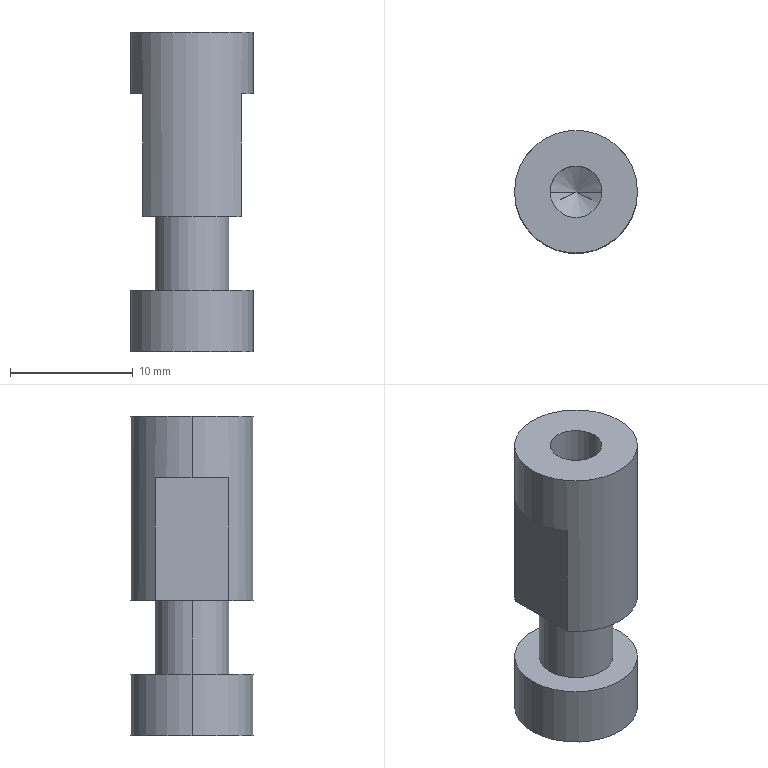Part | STEP file | 2100 Cylinder joint | 1 solid | 18 faces | box 10 x 10 x 26 mm | volume 1459 mm3 | cylinder 8 | plane 8 | cone 2 | commonest cylinder face diameters 10 x4 4.2 x2 6 x2
STEP:
#1=CARTESIAN_POINT('',(0.,0.,0.));
#2=DIRECTION('',(0.,0.,1.));
#3=DIRECTION('',(1.,0.,0.));
#4=AXIS2_PLACEMENT_3D('',#1,#2,#3);
#5=CARTESIAN_POINT('',(2.1,0.,12.));
#6=VERTEX_POINT('',#5);
#7=CARTESIAN_POINT('',(2.1,0.,26.));
#8=VERTEX_POINT('',#7);
#9=CARTESIAN_POINT('',(2.1,0.,26.));
#10=DIRECTION('',(0.,0.,1.));
#11=VECTOR('',#10,1.);
#12=LINE('',#9,#11);
#13=CARTESIAN_POINT('',(0.,0.,26.));
#14=DIRECTION('',(0.,0.,1.));
#15=DIRECTION('',(1.,0.,0.));
#16=AXIS2_PLACEMENT_3D('',#13,#14,#15);
#17=CYLINDRICAL_SURFACE('',#16,2.1);
#18=CARTESIAN_POINT('',(6.283,0.));
#19=DIRECTION('',(0.,1.));
#20=VECTOR('',#19,1.);
#21=LINE('',#18,#20);
#22=(GEOMETRIC_REPRESENTATION_CONTEXT(2)PARAMETRIC_REPRESENTATION_CONTEXT()REPRESENTATION_CONTEXT('',''));
#23=DEFINITIONAL_REPRESENTATION('',(#21),#22);
#24=PCURVE('',#17,#23);
#25=CARTESIAN_POINT('',(0.,0.,26.));
#26=DIRECTION('',(0.,0.,1.));
#27=DIRECTION('',(1.,0.,0.));
#28=AXIS2_PLACEMENT_3D('',#25,#26,#27);
#29=CYLINDRICAL_SURFACE('',#28,2.1);
#30=CARTESIAN_POINT('',(0.,0.));
#31=DIRECTION('',(0.,1.));
#32=VECTOR('',#31,1.);
#33=LINE('',#30,#32);
#34=(GEOMETRIC_REPRESENTATION_CONTEXT(2)PARAMETRIC_REPRESENTATION_CONTEXT()REPRESENTATION_CONTEXT('',''));
#35=DEFINITIONAL_REPRESENTATION('',(#33),#34);
#36=PCURVE('',#29,#35);
#37=SURFACE_CURVE('',#12,(#24,#36),.PCURVE_S1.);
#38=EDGE_CURVE('',#6,#8,#37,.T.);
#39=ORIENTED_EDGE('',*,*,#38,.T.);
#40=CARTESIAN_POINT('',(-2.1,0.,26.));
#41=VERTEX_POINT('',#40);
#42=CARTESIAN_POINT('',(0.,0.,26.));
#43=DIRECTION('',(0.,0.,1.));
#44=DIRECTION('',(1.,0.,0.));
#45=AXIS2_PLACEMENT_3D('',#42,#43,#44);
#46=CIRCLE('',#45,2.1);
#47=CARTESIAN_POINT('',(0.,0.));
#48=DIRECTION('',(1.,0.));
#49=VECTOR('',#48,1.);
#50=LINE('',#47,#49);
#51=(GEOMETRIC_REPRESENTATION_CONTEXT(2)PARAMETRIC_REPRESENTATION_CONTEXT()REPRESENTATION_CONTEXT('',''));
#52=DEFINITIONAL_REPRESENTATION('',(#50),#51);
#53=PCURVE('',#17,#52);
#54=CARTESIAN_POINT('',(0.,0.,26.));
#55=DIRECTION('',(0.,0.,1.));
#56=DIRECTION('',(1.,0.,0.));
#57=AXIS2_PLACEMENT_3D('',#54,#55,#56);
#58=PLANE('',#57);
#59=CARTESIAN_POINT('',(0.,0.));
#60=DIRECTION('',(1.,0.));
#61=AXIS2_PLACEMENT_2D('',#59,#60);
#62=CIRCLE('',#61,2.1);
#63=(GEOMETRIC_REPRESENTATION_CONTEXT(2)PARAMETRIC_REPRESENTATION_CONTEXT()REPRESENTATION_CONTEXT('',''));
#64=DEFINITIONAL_REPRESENTATION('',(#62),#63);
#65=PCURVE('',#58,#64);
#66=SURFACE_CURVE('',#46,(#53,#65),.PCURVE_S1.);
#67=EDGE_CURVE('',#41,#8,#66,.T.);
#68=ORIENTED_EDGE('',*,*,#67,.F.);
#69=CARTESIAN_POINT('',(-2.1,0.,12.));
#70=VERTEX_POINT('',#69);
#71=CARTESIAN_POINT('',(-2.1,0.,26.));
#72=DIRECTION('',(0.,0.,1.));
#73=VECTOR('',#72,1.);
#74=LINE('',#71,#73);
#75=CARTESIAN_POINT('',(3.142,0.));
#76=DIRECTION('',(0.,1.));
#77=VECTOR('',#76,1.);
#78=LINE('',#75,#77);
#79=(GEOMETRIC_REPRESENTATION_CONTEXT(2)PARAMETRIC_REPRESENTATION_CONTEXT()REPRESENTATION_CONTEXT('',''));
#80=DEFINITIONAL_REPRESENTATION('',(#78),#79);
#81=PCURVE('',#17,#80);
#82=CARTESIAN_POINT('',(3.142,0.));
#83=DIRECTION('',(0.,1.));
#84=VECTOR('',#83,1.);
#85=LINE('',#82,#84);
#86=(GEOMETRIC_REPRESENTATION_CONTEXT(2)PARAMETRIC_REPRESENTATION_CONTEXT()REPRESENTATION_CONTEXT('',''));
#87=DEFINITIONAL_REPRESENTATION('',(#85),#86);
#88=PCURVE('',#29,#87);
#89=SURFACE_CURVE('',#74,(#81,#88),.PCURVE_S1.);
#90=EDGE_CURVE('',#70,#41,#89,.T.);
#91=ORIENTED_EDGE('',*,*,#90,.F.);
#92=CARTESIAN_POINT('',(0.,0.,12.));
#93=DIRECTION('',(0.,0.,1.));
#94=DIRECTION('',(1.,0.,0.));
#95=AXIS2_PLACEMENT_3D('',#92,#93,#94);
#96=CIRCLE('',#95,2.1);
#97=CARTESIAN_POINT('',(0.,-14.));
#98=DIRECTION('',(1.,0.));
#99=VECTOR('',#98,1.);
#100=LINE('',#97,#99);
#101=(GEOMETRIC_REPRESENTATION_CONTEXT(2)PARAMETRIC_REPRESENTATION_CONTEXT()REPRESENTATION_CONTEXT('',''));
#102=DEFINITIONAL_REPRESENTATION('',(#100),#101);
#103=PCURVE('',#17,#102);
#104=CARTESIAN_POINT('',(0.,0.,12.));
#105=DIRECTION('',(0.,0.,1.));
#106=DIRECTION('',(1.,0.,0.));
#107=AXIS2_PLACEMENT_3D('',#104,#105,#106);
#108=CONICAL_SURFACE('',#107,2.1,1.03);
#109=CARTESIAN_POINT('',(0.,0.));
#110=DIRECTION('',(1.,0.));
#111=VECTOR('',#110,1.);
#112=LINE('',#109,#111);
#113=(GEOMETRIC_REPRESENTATION_CONTEXT(2)PARAMETRIC_REPRESENTATION_CONTEXT()REPRESENTATION_CONTEXT('',''));
#114=DEFINITIONAL_REPRESENTATION('',(#112),#113);
#115=PCURVE('',#108,#114);
#116=SURFACE_CURVE('',#96,(#103,#115),.PCURVE_S1.);
#117=EDGE_CURVE('',#70,#6,#116,.T.);
#118=ORIENTED_EDGE('',*,*,#117,.T.);
#119=EDGE_LOOP('',(#39,#68,#91,#118));
#120=FACE_BOUND('',#119,.F.);
#121=ADVANCED_FACE('',(#120),#17,.F.);
#122=ORIENTED_EDGE('',*,*,#117,.F.);
#123=CARTESIAN_POINT('',(0.,0.,10.738));
#124=VERTEX_POINT('',#123);
#125=CARTESIAN_POINT('',(-2.1,0.,12.));
#126=DIRECTION('',(-0.8572,0.,0.515));
#127=VECTOR('',#126,1.);
#128=LINE('',#125,#127);
#129=CARTESIAN_POINT('',(3.142,0.));
#130=DIRECTION('',(0.,1.));
#131=VECTOR('',#130,1.);
#132=LINE('',#129,#131);
#133=(GEOMETRIC_REPRESENTATION_CONTEXT(2)PARAMETRIC_REPRESENTATION_CONTEXT()REPRESENTATION_CONTEXT('',''));
#134=DEFINITIONAL_REPRESENTATION('',(#132),#133);
#135=PCURVE('',#108,#134);
#136=CARTESIAN_POINT('',(0.,0.,12.));
#137=DIRECTION('',(0.,0.,1.));
#138=DIRECTION('',(1.,0.,0.));
#139=AXIS2_PLACEMENT_3D('',#136,#137,#138);
#140=CONICAL_SURFACE('',#139,2.1,1.03);
#141=CARTESIAN_POINT('',(3.142,0.));
#142=DIRECTION('',(0.,1.));
#143=VECTOR('',#142,1.);
#144=LINE('',#141,#143);
#145=(GEOMETRIC_REPRESENTATION_CONTEXT(2)PARAMETRIC_REPRESENTATION_CONTEXT()REPRESENTATION_CONTEXT('',''));
#146=DEFINITIONAL_REPRESENTATION('',(#144),#145);
#147=PCURVE('',#140,#146);
#148=SURFACE_CURVE('',#128,(#135,#147),.PCURVE_S1.);
#149=EDGE_CURVE('',#124,#70,#148,.T.);
#150=ORIENTED_EDGE('',*,*,#149,.F.);
#151=CARTESIAN_POINT('',(2.1,0.,12.));
#152=DIRECTION('',(0.8572,0.,0.515));
#153=VECTOR('',#152,1.);
#154=LINE('',#151,#153);
#155=CARTESIAN_POINT('',(6.283,0.));
#156=DIRECTION('',(0.,1.));
#157=VECTOR('',#156,1.);
#158=LINE('',#155,#157);
#159=(GEOMETRIC_REPRESENTATION_CONTEXT(2)PARAMETRIC_REPRESENTATION_CONTEXT()REPRESENTATION_CONTEXT('',''));
#160=DEFINITIONAL_REPRESENTATION('',(#158),#159);
#161=PCURVE('',#108,#160);
#162=CARTESIAN_POINT('',(0.,0.));
#163=DIRECTION('',(0.,1.));
#164=VECTOR('',#163,1.);
#165=LINE('',#162,#164);
#166=(GEOMETRIC_REPRESENTATION_CONTEXT(2)PARAMETRIC_REPRESENTATION_CONTEXT()REPRESENTATION_CONTEXT('',''));
#167=DEFINITIONAL_REPRESENTATION('',(#165),#166);
#168=PCURVE('',#140,#167);
#169=SURFACE_CURVE('',#154,(#161,#168),.PCURVE_S1.);
#170=EDGE_CURVE('',#124,#6,#169,.T.);
#171=ORIENTED_EDGE('',*,*,#170,.T.);
#172=EDGE_LOOP('',(#122,#150,#171));
#173=FACE_BOUND('',#172,.F.);
#174=ADVANCED_FACE('',(#173),#108,.F.);
#175=CARTESIAN_POINT('',(3.,0.,11.));
#176=VERTEX_POINT('',#175);
#177=CARTESIAN_POINT('',(-3.,0.,11.));
#178=VERTEX_POINT('',#177);
#179=CARTESIAN_POINT('',(0.,0.,11.));
#180=DIRECTION('',(0.,0.,1.));
#181=DIRECTION('',(1.,0.,0.));
#182=AXIS2_PLACEMENT_3D('',#179,#180,#181);
#183=CIRCLE('',#182,3.);
#184=CARTESIAN_POINT('',(0.,0.,11.));
#185=DIRECTION('',(0.,0.,-1.));
#186=DIRECTION('',(-1.,0.,0.));
#187=AXIS2_PLACEMENT_3D('',#184,#185,#186);
#188=CYLINDRICAL_SURFACE('',#187,3.);
#189=CARTESIAN_POINT('',(3.142,0.));
#190=DIRECTION('',(-1.,0.));
#191=VECTOR('',#190,1.);
#192=LINE('',#189,#191);
#193=(GEOMETRIC_REPRESENTATION_CONTEXT(2)PARAMETRIC_REPRESENTATION_CONTEXT()REPRESENTATION_CONTEXT('',''));
#194=DEFINITIONAL_REPRESENTATION('',(#192),#193);
#195=PCURVE('',#188,#194);
#196=CARTESIAN_POINT('',(0.,0.,11.));
#197=DIRECTION('',(0.,0.,1.));
#198=DIRECTION('',(1.,0.,0.));
#199=AXIS2_PLACEMENT_3D('',#196,#197,#198);
#200=PLANE('',#199);
#201=CARTESIAN_POINT('',(0.,0.));
#202=DIRECTION('',(1.,0.));
#203=AXIS2_PLACEMENT_2D('',#201,#202);
#204=CIRCLE('',#203,3.);
#205=(GEOMETRIC_REPRESENTATION_CONTEXT(2)PARAMETRIC_REPRESENTATION_CONTEXT()REPRESENTATION_CONTEXT('',''));
#206=DEFINITIONAL_REPRESENTATION('',(#204),#205);
#207=PCURVE('',#200,#206);
#208=SURFACE_CURVE('',#183,(#195,#207),.PCURVE_S1.);
#209=EDGE_CURVE('',#176,#178,#208,.T.);
#210=ORIENTED_EDGE('',*,*,#209,.F.);
#211=CARTESIAN_POINT('',(3.,0.,5.));
#212=VERTEX_POINT('',#211);
#213=CARTESIAN_POINT('',(3.,0.,11.));
#214=DIRECTION('',(0.,0.,-1.));
#215=VECTOR('',#214,1.);
#216=LINE('',#213,#215);
#217=CARTESIAN_POINT('',(3.142,0.));
#218=DIRECTION('',(0.,1.));
#219=VECTOR('',#218,1.);
#220=LINE('',#217,#219);
#221=(GEOMETRIC_REPRESENTATION_CONTEXT(2)PARAMETRIC_REPRESENTATION_CONTEXT()REPRESENTATION_CONTEXT('',''));
#222=DEFINITIONAL_REPRESENTATION('',(#220),#221);
#223=PCURVE('',#188,#222);
#224=CARTESIAN_POINT('',(0.,0.,11.));
#225=DIRECTION('',(0.,0.,-1.));
#226=DIRECTION('',(-1.,0.,0.));
#227=AXIS2_PLACEMENT_3D('',#224,#225,#226);
#228=CYLINDRICAL_SURFACE('',#227,3.);
#229=CARTESIAN_POINT('',(3.142,0.));
#230=DIRECTION('',(0.,1.));
#231=VECTOR('',#230,1.);
#232=LINE('',#229,#231);
#233=(GEOMETRIC_REPRESENTATION_CONTEXT(2)PARAMETRIC_REPRESENTATION_CONTEXT()REPRESENTATION_CONTEXT('',''));
#234=DEFINITIONAL_REPRESENTATION('',(#232),#233);
#235=PCURVE('',#228,#234);
#236=SURFACE_CURVE('',#216,(#223,#235),.PCURVE_S1.);
#237=EDGE_CURVE('',#176,#212,#236,.T.);
#238=ORIENTED_EDGE('',*,*,#237,.T.);
#239=CARTESIAN_POINT('',(-3.,0.,5.));
#240=VERTEX_POINT('',#239);
#241=CARTESIAN_POINT('',(0.,0.,5.));
#242=DIRECTION('',(0.,0.,1.));
#243=DIRECTION('',(1.,0.,0.));
#244=AXIS2_PLACEMENT_3D('',#241,#242,#243);
#245=CIRCLE('',#244,3.);
#246=CARTESIAN_POINT('',(3.142,6.));
#247=DIRECTION('',(-1.,0.));
#248=VECTOR('',#247,1.);
#249=LINE('',#246,#248);
#250=(GEOMETRIC_REPRESENTATION_CONTEXT(2)PARAMETRIC_REPRESENTATION_CONTEXT()REPRESENTATION_CONTEXT('',''));
#251=DEFINITIONAL_REPRESENTATION('',(#249),#250);
#252=PCURVE('',#188,#251);
#253=CARTESIAN_POINT('',(0.,0.,5.));
#254=DIRECTION('',(0.,0.,1.));
#255=DIRECTION('',(1.,0.,0.));
#256=AXIS2_PLACEMENT_3D('',#253,#254,#255);
#257=PLANE('',#256);
#258=CARTESIAN_POINT('',(0.,0.));
#259=DIRECTION('',(1.,0.));
#260=AXIS2_PLACEMENT_2D('',#258,#259);
#261=CIRCLE('',#260,3.);
#262=(GEOMETRIC_REPRESENTATION_CONTEXT(2)PARAMETRIC_REPRESENTATION_CONTEXT()REPRESENTATION_CONTEXT('',''));
#263=DEFINITIONAL_REPRESENTATION('',(#261),#262);
#264=PCURVE('',#257,#263);
#265=SURFACE_CURVE('',#245,(#252,#264),.PCURVE_S1.);
#266=EDGE_CURVE('',#212,#240,#265,.T.);
#267=ORIENTED_EDGE('',*,*,#266,.T.);
#268=CARTESIAN_POINT('',(-3.,0.,11.));
#269=DIRECTION('',(0.,0.,-1.));
#270=VECTOR('',#269,1.);
#271=LINE('',#268,#270);
#272=CARTESIAN_POINT('',(0.,0.));
#273=DIRECTION('',(0.,1.));
#274=VECTOR('',#273,1.);
#275=LINE('',#272,#274);
#276=(GEOMETRIC_REPRESENTATION_CONTEXT(2)PARAMETRIC_REPRESENTATION_CONTEXT()REPRESENTATION_CONTEXT('',''));
#277=DEFINITIONAL_REPRESENTATION('',(#275),#276);
#278=PCURVE('',#188,#277);
#279=CARTESIAN_POINT('',(6.283,0.));
#280=DIRECTION('',(0.,1.));
#281=VECTOR('',#280,1.);
#282=LINE('',#279,#281);
#283=(GEOMETRIC_REPRESENTATION_CONTEXT(2)PARAMETRIC_REPRESENTATION_CONTEXT()REPRESENTATION_CONTEXT('',''));
#284=DEFINITIONAL_REPRESENTATION('',(#282),#283);
#285=PCURVE('',#228,#284);
#286=SURFACE_CURVE('',#271,(#278,#285),.PCURVE_S1.);
#287=EDGE_CURVE('',#178,#240,#286,.T.);
#288=ORIENTED_EDGE('',*,*,#287,.F.);
#289=EDGE_LOOP('',(#210,#238,#267,#288));
#290=FACE_BOUND('',#289,.T.);
#291=ADVANCED_FACE('',(#290),#188,.T.);
#292=CARTESIAN_POINT('',(5.,0.,5.));
#293=VERTEX_POINT('',#292);
#294=CARTESIAN_POINT('',(-5.,0.,5.));
#295=VERTEX_POINT('',#294);
#296=CARTESIAN_POINT('',(0.,0.,5.));
#297=DIRECTION('',(0.,0.,1.));
#298=DIRECTION('',(1.,0.,0.));
#299=AXIS2_PLACEMENT_3D('',#296,#297,#298);
#300=CIRCLE('',#299,5.);
#301=CARTESIAN_POINT('',(0.,0.,5.));
#302=DIRECTION('',(0.,0.,-1.));
#303=DIRECTION('',(-1.,0.,0.));
#304=AXIS2_PLACEMENT_3D('',#301,#302,#303);
#305=CYLINDRICAL_SURFACE('',#304,5.);
#306=CARTESIAN_POINT('',(3.142,0.));
#307=DIRECTION('',(-1.,0.));
#308=VECTOR('',#307,1.);
#309=LINE('',#306,#308);
#310=(GEOMETRIC_REPRESENTATION_CONTEXT(2)PARAMETRIC_REPRESENTATION_CONTEXT()REPRESENTATION_CONTEXT('',''));
#311=DEFINITIONAL_REPRESENTATION('',(#309),#310);
#312=PCURVE('',#305,#311);
#313=CARTESIAN_POINT('',(0.,0.));
#314=DIRECTION('',(1.,0.));
#315=AXIS2_PLACEMENT_2D('',#313,#314);
#316=CIRCLE('',#315,5.);
#317=(GEOMETRIC_REPRESENTATION_CONTEXT(2)PARAMETRIC_REPRESENTATION_CONTEXT()REPRESENTATION_CONTEXT('',''));
#318=DEFINITIONAL_REPRESENTATION('',(#316),#317);
#319=PCURVE('',#257,#318);
#320=SURFACE_CURVE('',#300,(#312,#319),.PCURVE_S1.);
#321=EDGE_CURVE('',#293,#295,#320,.T.);
#322=ORIENTED_EDGE('',*,*,#321,.F.);
#323=CARTESIAN_POINT('',(5.,0.,0.));
#324=VERTEX_POINT('',#323);
#325=CARTESIAN_POINT('',(5.,0.,5.));
#326=DIRECTION('',(0.,0.,-1.));
#327=VECTOR('',#326,1.);
#328=LINE('',#325,#327);
#329=CARTESIAN_POINT('',(3.142,0.));
#330=DIRECTION('',(0.,1.));
#331=VECTOR('',#330,1.);
#332=LINE('',#329,#331);
#333=(GEOMETRIC_REPRESENTATION_CONTEXT(2)PARAMETRIC_REPRESENTATION_CONTEXT()REPRESENTATION_CONTEXT('',''));
#334=DEFINITIONAL_REPRESENTATION('',(#332),#333);
#335=PCURVE('',#305,#334);
#336=CARTESIAN_POINT('',(0.,0.,5.));
#337=DIRECTION('',(0.,0.,-1.));
#338=DIRECTION('',(-1.,0.,0.));
#339=AXIS2_PLACEMENT_3D('',#336,#337,#338);
#340=CYLINDRICAL_SURFACE('',#339,5.);
#341=CARTESIAN_POINT('',(3.142,0.));
#342=DIRECTION('',(0.,1.));
#343=VECTOR('',#342,1.);
#344=LINE('',#341,#343);
#345=(GEOMETRIC_REPRESENTATION_CONTEXT(2)PARAMETRIC_REPRESENTATION_CONTEXT()REPRESENTATION_CONTEXT('',''));
#346=DEFINITIONAL_REPRESENTATION('',(#344),#345);
#347=PCURVE('',#340,#346);
#348=SURFACE_CURVE('',#328,(#335,#347),.PCURVE_S1.);
#349=EDGE_CURVE('',#293,#324,#348,.T.);
#350=ORIENTED_EDGE('',*,*,#349,.T.);
#351=CARTESIAN_POINT('',(-5.,0.,0.));
#352=VERTEX_POINT('',#351);
#353=CARTESIAN_POINT('',(0.,0.,0.));
#354=DIRECTION('',(0.,0.,1.));
#355=DIRECTION('',(1.,0.,0.));
#356=AXIS2_PLACEMENT_3D('',#353,#354,#355);
#357=CIRCLE('',#356,5.);
#358=CARTESIAN_POINT('',(3.142,5.));
#359=DIRECTION('',(-1.,0.));
#360=VECTOR('',#359,1.);
#361=LINE('',#358,#360);
#362=(GEOMETRIC_REPRESENTATION_CONTEXT(2)PARAMETRIC_REPRESENTATION_CONTEXT()REPRESENTATION_CONTEXT('',''));
#363=DEFINITIONAL_REPRESENTATION('',(#361),#362);
#364=PCURVE('',#305,#363);
#365=CARTESIAN_POINT('',(0.,0.,0.));
#366=DIRECTION('',(0.,0.,1.));
#367=DIRECTION('',(1.,0.,0.));
#368=AXIS2_PLACEMENT_3D('',#365,#366,#367);
#369=PLANE('',#368);
#370=CARTESIAN_POINT('',(0.,0.));
#371=DIRECTION('',(1.,0.));
#372=AXIS2_PLACEMENT_2D('',#370,#371);
#373=CIRCLE('',#372,5.);
#374=(GEOMETRIC_REPRESENTATION_CONTEXT(2)PARAMETRIC_REPRESENTATION_CONTEXT()REPRESENTATION_CONTEXT('',''));
#375=DEFINITIONAL_REPRESENTATION('',(#373),#374);
#376=PCURVE('',#369,#375);
#377=SURFACE_CURVE('',#357,(#364,#376),.PCURVE_S1.);
#378=EDGE_CURVE('',#324,#352,#377,.T.);
#379=ORIENTED_EDGE('',*,*,#378,.T.);
#380=CARTESIAN_POINT('',(-5.,0.,5.));
#381=DIRECTION('',(0.,0.,-1.));
#382=VECTOR('',#381,1.);
#383=LINE('',#380,#382);
#384=CARTESIAN_POINT('',(0.,0.));
#385=DIRECTION('',(0.,1.));
#386=VECTOR('',#385,1.);
#387=LINE('',#384,#386);
#388=(GEOMETRIC_REPRESENTATION_CONTEXT(2)PARAMETRIC_REPRESENTATION_CONTEXT()REPRESENTATION_CONTEXT('',''));
#389=DEFINITIONAL_REPRESENTATION('',(#387),#388);
#390=PCURVE('',#305,#389);
#391=CARTESIAN_POINT('',(6.283,0.));
#392=DIRECTION('',(0.,1.));
#393=VECTOR('',#392,1.);
#394=LINE('',#391,#393);
#395=(GEOMETRIC_REPRESENTATION_CONTEXT(2)PARAMETRIC_REPRESENTATION_CONTEXT()REPRESENTATION_CONTEXT('',''));
#396=DEFINITIONAL_REPRESENTATION('',(#394),#395);
#397=PCURVE('',#340,#396);
#398=SURFACE_CURVE('',#383,(#390,#397),.PCURVE_S1.);
#399=EDGE_CURVE('',#295,#352,#398,.T.);
#400=ORIENTED_EDGE('',*,*,#399,.F.);
#401=EDGE_LOOP('',(#322,#350,#379,#400));
#402=FACE_BOUND('',#401,.T.);
#403=ADVANCED_FACE('',(#402),#305,.T.);
#404=CARTESIAN_POINT('',(5.,0.,26.));
#405=VERTEX_POINT('',#404);
#406=CARTESIAN_POINT('',(-5.,0.,26.));
#407=VERTEX_POINT('',#406);
#408=CARTESIAN_POINT('',(0.,0.,26.));
#409=DIRECTION('',(0.,0.,1.));
#410=DIRECTION('',(1.,0.,0.));
#411=AXIS2_PLACEMENT_3D('',#408,#409,#410);
#412=CIRCLE('',#411,5.);
#413=CARTESIAN_POINT('',(0.,0.,26.));
#414=DIRECTION('',(0.,0.,-1.));
#415=DIRECTION('',(-1.,0.,0.));
#416=AXIS2_PLACEMENT_3D('',#413,#414,#415);
#417=CYLINDRICAL_SURFACE('',#416,5.);
#418=CARTESIAN_POINT('',(3.142,0.));
#419=DIRECTION('',(-1.,0.));
#420=VECTOR('',#419,1.);
#421=LINE('',#418,#420);
#422=(GEOMETRIC_REPRESENTATION_CONTEXT(2)PARAMETRIC_REPRESENTATION_CONTEXT()REPRESENTATION_CONTEXT('',''));
#423=DEFINITIONAL_REPRESENTATION('',(#421),#422);
#424=PCURVE('',#417,#423);
#425=CARTESIAN_POINT('',(0.,0.));
#426=DIRECTION('',(1.,0.));
#427=AXIS2_PLACEMENT_2D('',#425,#426);
#428=CIRCLE('',#427,5.);
#429=(GEOMETRIC_REPRESENTATION_CONTEXT(2)PARAMETRIC_REPRESENTATION_CONTEXT()REPRESENTATION_CONTEXT('',''));
#430=DEFINITIONAL_REPRESENTATION('',(#428),#429);
#431=PCURVE('',#58,#430);
#432=SURFACE_CURVE('',#412,(#424,#431),.PCURVE_S1.);
#433=EDGE_CURVE('',#405,#407,#432,.T.);
#434=ORIENTED_EDGE('',*,*,#433,.F.);
#435=CARTESIAN_POINT('',(5.,0.,21.));
#436=VERTEX_POINT('',#435);
#437=CARTESIAN_POINT('',(5.,0.,26.));
#438=DIRECTION('',(0.,0.,-1.));
#439=VECTOR('',#438,1.);
#440=LINE('',#437,#439);
#441=CARTESIAN_POINT('',(3.142,0.));
#442=DIRECTION('',(0.,1.));
#443=VECTOR('',#442,1.);
#444=LINE('',#441,#443);
#445=(GEOMETRIC_REPRESENTATION_CONTEXT(2)PARAMETRIC_REPRESENTATION_CONTEXT()REPRESENTATION_CONTEXT('',''));
#446=DEFINITIONAL_REPRESENTATION('',(#444),#445);
#447=PCURVE('',#417,#446);
#448=CARTESIAN_POINT('',(0.,0.,26.));
#449=DIRECTION('',(0.,0.,-1.));
#450=DIRECTION('',(-1.,0.,0.));
#451=AXIS2_PLACEMENT_3D('',#448,#449,#450);
#452=CYLINDRICAL_SURFACE('',#451,5.);
#453=CARTESIAN_POINT('',(3.142,0.));
#454=DIRECTION('',(0.,1.));
#455=VECTOR('',#454,1.);
#456=LINE('',#453,#455);
#457=(GEOMETRIC_REPRESENTATION_CONTEXT(2)PARAMETRIC_REPRESENTATION_CONTEXT()REPRESENTATION_CONTEXT('',''));
#458=DEFINITIONAL_REPRESENTATION('',(#456),#457);
#459=PCURVE('',#452,#458);
#460=SURFACE_CURVE('',#440,(#447,#459),.PCURVE_S1.);
#461=EDGE_CURVE('',#405,#436,#460,.T.);
#462=ORIENTED_EDGE('',*,*,#461,.T.);
#463=CARTESIAN_POINT('',(4.,3.,21.));
#464=VERTEX_POINT('',#463);
#465=CARTESIAN_POINT('',(0.,0.,21.));
#466=DIRECTION('',(0.,0.,-1.));
#467=DIRECTION('',(-1.,0.,0.));
#468=AXIS2_PLACEMENT_3D('',#465,#466,#467);
#469=CIRCLE('',#468,5.);
#470=CARTESIAN_POINT('',(0.,5.));
#471=DIRECTION('',(1.,0.));
#472=VECTOR('',#471,1.);
#473=LINE('',#470,#472);
#474=(GEOMETRIC_REPRESENTATION_CONTEXT(2)PARAMETRIC_REPRESENTATION_CONTEXT()REPRESENTATION_CONTEXT('',''));
#475=DEFINITIONAL_REPRESENTATION('',(#473),#474);
#476=PCURVE('',#417,#475);
#477=CARTESIAN_POINT('',(11.893,50.,21.));
#478=DIRECTION('',(0.,0.,-1.));
#479=DIRECTION('',(-1.,0.,0.));
#480=AXIS2_PLACEMENT_3D('',#477,#478,#479);
#481=PLANE('',#480);
#482=CARTESIAN_POINT('',(11.893,-50.));
#483=DIRECTION('',(1.,0.));
#484=AXIS2_PLACEMENT_2D('',#482,#483);
#485=CIRCLE('',#484,5.);
#486=(GEOMETRIC_REPRESENTATION_CONTEXT(2)PARAMETRIC_REPRESENTATION_CONTEXT()REPRESENTATION_CONTEXT('',''));
#487=DEFINITIONAL_REPRESENTATION('',(#485),#486);
#488=PCURVE('',#481,#487);
#489=SURFACE_CURVE('',#469,(#476,#488),.PCURVE_S1.);
#490=EDGE_CURVE('',#464,#436,#489,.T.);
#491=ORIENTED_EDGE('',*,*,#490,.F.);
#492=CARTESIAN_POINT('',(4.,3.,11.));
#493=VERTEX_POINT('',#492);
#494=CARTESIAN_POINT('',(4.,3.,26.));
#495=DIRECTION('',(0.,0.,1.));
#496=VECTOR('',#495,1.);
#497=LINE('',#494,#496);
#498=CARTESIAN_POINT('',(2.498,0.));
#499=DIRECTION('',(0.,-1.));
#500=VECTOR('',#499,1.);
#501=LINE('',#498,#500);
#502=(GEOMETRIC_REPRESENTATION_CONTEXT(2)PARAMETRIC_REPRESENTATION_CONTEXT()REPRESENTATION_CONTEXT('',''));
#503=DEFINITIONAL_REPRESENTATION('',(#501),#502);
#504=PCURVE('',#417,#503);
#505=CARTESIAN_POINT('',(4.,50.,9.));
#506=DIRECTION('',(1.,0.,0.));
#507=DIRECTION('',(0.,0.,-1.));
#508=AXIS2_PLACEMENT_3D('',#505,#506,#507);
#509=PLANE('',#508);
#510=CARTESIAN_POINT('',(-17.,-47.));
#511=DIRECTION('',(-1.,0.));
#512=VECTOR('',#511,1.);
#513=LINE('',#510,#512);
#514=(GEOMETRIC_REPRESENTATION_CONTEXT(2)PARAMETRIC_REPRESENTATION_CONTEXT()REPRESENTATION_CONTEXT('',''));
#515=DEFINITIONAL_REPRESENTATION('',(#513),#514);
#516=PCURVE('',#509,#515);
#517=SURFACE_CURVE('',#497,(#504,#516),.PCURVE_S1.);
#518=EDGE_CURVE('',#493,#464,#517,.T.);
#519=ORIENTED_EDGE('',*,*,#518,.F.);
#520=CARTESIAN_POINT('',(-4.,3.,11.));
#521=VERTEX_POINT('',#520);
#522=CARTESIAN_POINT('',(0.,0.,11.));
#523=DIRECTION('',(0.,0.,1.));
#524=DIRECTION('',(1.,0.,0.));
#525=AXIS2_PLACEMENT_3D('',#522,#523,#524);
#526=CIRCLE('',#525,5.);
#527=CARTESIAN_POINT('',(3.142,15.));
#528=DIRECTION('',(-1.,0.));
#529=VECTOR('',#528,1.);
#530=LINE('',#527,#529);
#531=(GEOMETRIC_REPRESENTATION_CONTEXT(2)PARAMETRIC_REPRESENTATION_CONTEXT()REPRESENTATION_CONTEXT('',''));
#532=DEFINITIONAL_REPRESENTATION('',(#530),#531);
#533=PCURVE('',#417,#532);
#534=CARTESIAN_POINT('',(0.,0.));
#535=DIRECTION('',(1.,0.));
#536=AXIS2_PLACEMENT_2D('',#534,#535);
#537=CIRCLE('',#536,5.);
#538=(GEOMETRIC_REPRESENTATION_CONTEXT(2)PARAMETRIC_REPRESENTATION_CONTEXT()REPRESENTATION_CONTEXT('',''));
#539=DEFINITIONAL_REPRESENTATION('',(#537),#538);
#540=PCURVE('',#200,#539);
#541=SURFACE_CURVE('',#526,(#533,#540),.PCURVE_S1.);
#542=EDGE_CURVE('',#493,#521,#541,.T.);
#543=ORIENTED_EDGE('',*,*,#542,.T.);
#544=CARTESIAN_POINT('',(-4.,3.,21.));
#545=VERTEX_POINT('',#544);
#546=CARTESIAN_POINT('',(-4.,3.,26.));
#547=DIRECTION('',(0.,0.,-1.));
#548=VECTOR('',#547,1.);
#549=LINE('',#546,#548);
#550=CARTESIAN_POINT('',(0.6435,0.));
#551=DIRECTION('',(0.,1.));
#552=VECTOR('',#551,1.);
#553=LINE('',#550,#552);
#554=(GEOMETRIC_REPRESENTATION_CONTEXT(2)PARAMETRIC_REPRESENTATION_CONTEXT()REPRESENTATION_CONTEXT('',''));
#555=DEFINITIONAL_REPRESENTATION('',(#553),#554);
#556=PCURVE('',#417,#555);
#557=CARTESIAN_POINT('',(-4.,50.,9.));
#558=DIRECTION('',(-1.,0.,0.));
#559=DIRECTION('',(0.,0.,1.));
#560=AXIS2_PLACEMENT_3D('',#557,#558,#559);
#561=PLANE('',#560);
#562=CARTESIAN_POINT('',(17.,-47.));
#563=DIRECTION('',(-1.,0.));
#564=VECTOR('',#563,1.);
#565=LINE('',#562,#564);
#566=(GEOMETRIC_REPRESENTATION_CONTEXT(2)PARAMETRIC_REPRESENTATION_CONTEXT()REPRESENTATION_CONTEXT('',''));
#567=DEFINITIONAL_REPRESENTATION('',(#565),#566);
#568=PCURVE('',#561,#567);
#569=SURFACE_CURVE('',#549,(#556,#568),.PCURVE_S1.);
#570=EDGE_CURVE('',#545,#521,#569,.T.);
#571=ORIENTED_EDGE('',*,*,#570,.F.);
#572=CARTESIAN_POINT('',(-5.,0.,21.));
#573=VERTEX_POINT('',#572);
#574=CARTESIAN_POINT('',(0.,0.,21.));
#575=DIRECTION('',(0.,0.,-1.));
#576=DIRECTION('',(-1.,0.,0.));
#577=AXIS2_PLACEMENT_3D('',#574,#575,#576);
#578=CIRCLE('',#577,5.);
#579=CARTESIAN_POINT('',(0.,5.));
#580=DIRECTION('',(1.,0.));
#581=VECTOR('',#580,1.);
#582=LINE('',#579,#581);
#583=(GEOMETRIC_REPRESENTATION_CONTEXT(2)PARAMETRIC_REPRESENTATION_CONTEXT()REPRESENTATION_CONTEXT('',''));
#584=DEFINITIONAL_REPRESENTATION('',(#582),#583);
#585=PCURVE('',#417,#584);
#586=CARTESIAN_POINT('',(-11.893,50.,21.));
#587=DIRECTION('',(0.,0.,-1.));
#588=DIRECTION('',(-1.,0.,0.));
#589=AXIS2_PLACEMENT_3D('',#586,#587,#588);
#590=PLANE('',#589);
#591=CARTESIAN_POINT('',(-11.893,-50.));
#592=DIRECTION('',(1.,0.));
#593=AXIS2_PLACEMENT_2D('',#591,#592);
#594=CIRCLE('',#593,5.);
#595=(GEOMETRIC_REPRESENTATION_CONTEXT(2)PARAMETRIC_REPRESENTATION_CONTEXT()REPRESENTATION_CONTEXT('',''));
#596=DEFINITIONAL_REPRESENTATION('',(#594),#595);
#597=PCURVE('',#590,#596);
#598=SURFACE_CURVE('',#578,(#585,#597),.PCURVE_S1.);
#599=EDGE_CURVE('',#573,#545,#598,.T.);
#600=ORIENTED_EDGE('',*,*,#599,.F.);
#601=CARTESIAN_POINT('',(-5.,0.,26.));
#602=DIRECTION('',(0.,0.,-1.));
#603=VECTOR('',#602,1.);
#604=LINE('',#601,#603);
#605=CARTESIAN_POINT('',(0.,0.));
#606=DIRECTION('',(0.,1.));
#607=VECTOR('',#606,1.);
#608=LINE('',#605,#607);
#609=(GEOMETRIC_REPRESENTATION_CONTEXT(2)PARAMETRIC_REPRESENTATION_CONTEXT()REPRESENTATION_CONTEXT('',''));
#610=DEFINITIONAL_REPRESENTATION('',(#608),#609);
#611=PCURVE('',#417,#610);
#612=CARTESIAN_POINT('',(6.283,0.));
#613=DIRECTION('',(0.,1.));
#614=VECTOR('',#613,1.);
#615=LINE('',#612,#614);
#616=(GEOMETRIC_REPRESENTATION_CONTEXT(2)PARAMETRIC_REPRESENTATION_CONTEXT()REPRESENTATION_CONTEXT('',''));
#617=DEFINITIONAL_REPRESENTATION('',(#615),#616);
#618=PCURVE('',#452,#617);
#619=SURFACE_CURVE('',#604,(#611,#618),.PCURVE_S1.);
#620=EDGE_CURVE('',#407,#573,#619,.T.);
#621=ORIENTED_EDGE('',*,*,#620,.F.);
#622=EDGE_LOOP('',(#434,#462,#491,#519,#543,#571,#600,#621));
#623=FACE_BOUND('',#622,.T.);
#624=ADVANCED_FACE('',(#623),#417,.T.);
#625=CARTESIAN_POINT('',(0.,0.,11.));
#626=DIRECTION('',(0.,0.,1.));
#627=DIRECTION('',(1.,0.,0.));
#628=AXIS2_PLACEMENT_3D('',#625,#626,#627);
#629=CIRCLE('',#628,3.);
#630=CARTESIAN_POINT('',(0.,0.));
#631=DIRECTION('',(1.,0.));
#632=AXIS2_PLACEMENT_2D('',#630,#631);
#633=CIRCLE('',#632,3.);
#634=(GEOMETRIC_REPRESENTATION_CONTEXT(2)PARAMETRIC_REPRESENTATION_CONTEXT()REPRESENTATION_CONTEXT('',''));
#635=DEFINITIONAL_REPRESENTATION('',(#633),#634);
#636=PCURVE('',#200,#635);
#637=CARTESIAN_POINT('',(9.425,0.));
#638=DIRECTION('',(-1.,0.));
#639=VECTOR('',#638,1.);
#640=LINE('',#637,#639);
#641=(GEOMETRIC_REPRESENTATION_CONTEXT(2)PARAMETRIC_REPRESENTATION_CONTEXT()REPRESENTATION_CONTEXT('',''));
#642=DEFINITIONAL_REPRESENTATION('',(#640),#641);
#643=PCURVE('',#228,#642);
#644=SURFACE_CURVE('',#629,(#636,#643),.PCURVE_S1.);
#645=EDGE_CURVE('',#178,#176,#644,.T.);
#646=ORIENTED_EDGE('',*,*,#645,.T.);
#647=ORIENTED_EDGE('',*,*,#209,.T.);
#648=EDGE_LOOP('',(#646,#647));
#649=FACE_BOUND('',#648,.T.);
#650=CARTESIAN_POINT('',(4.,-3.,11.));
#651=VERTEX_POINT('',#650);
#652=CARTESIAN_POINT('',(4.,0.,11.));
#653=DIRECTION('',(0.,1.,0.));
#654=VECTOR('',#653,1.);
#655=LINE('',#652,#654);
#656=CARTESIAN_POINT('',(4.,0.));
#657=DIRECTION('',(0.,1.));
#658=VECTOR('',#657,1.);
#659=LINE('',#656,#658);
#660=(GEOMETRIC_REPRESENTATION_CONTEXT(2)PARAMETRIC_REPRESENTATION_CONTEXT()REPRESENTATION_CONTEXT('',''));
#661=DEFINITIONAL_REPRESENTATION('',(#659),#660);
#662=PCURVE('',#200,#661);
#663=CARTESIAN_POINT('',(-2.,-50.));
#664=DIRECTION('',(0.,1.));
#665=VECTOR('',#664,1.);
#666=LINE('',#663,#665);
#667=(GEOMETRIC_REPRESENTATION_CONTEXT(2)PARAMETRIC_REPRESENTATION_CONTEXT()REPRESENTATION_CONTEXT('',''));
#668=DEFINITIONAL_REPRESENTATION('',(#666),#667);
#669=PCURVE('',#509,#668);
#670=SURFACE_CURVE('',#655,(#662,#669),.PCURVE_S1.);
#671=EDGE_CURVE('',#651,#493,#670,.T.);
#672=ORIENTED_EDGE('',*,*,#671,.F.);
#673=CARTESIAN_POINT('',(-4.,-3.,11.));
#674=VERTEX_POINT('',#673);
#675=CARTESIAN_POINT('',(0.,0.,11.));
#676=DIRECTION('',(0.,0.,1.));
#677=DIRECTION('',(1.,0.,0.));
#678=AXIS2_PLACEMENT_3D('',#675,#676,#677);
#679=CIRCLE('',#678,5.);
#680=CARTESIAN_POINT('',(0.,0.));
#681=DIRECTION('',(1.,0.));
#682=AXIS2_PLACEMENT_2D('',#680,#681);
#683=CIRCLE('',#682,5.);
#684=(GEOMETRIC_REPRESENTATION_CONTEXT(2)PARAMETRIC_REPRESENTATION_CONTEXT()REPRESENTATION_CONTEXT('',''));
#685=DEFINITIONAL_REPRESENTATION('',(#683),#684);
#686=PCURVE('',#200,#685);
#687=CARTESIAN_POINT('',(9.425,15.));
#688=DIRECTION('',(-1.,0.));
#689=VECTOR('',#688,1.);
#690=LINE('',#687,#689);
#691=(GEOMETRIC_REPRESENTATION_CONTEXT(2)PARAMETRIC_REPRESENTATION_CONTEXT()REPRESENTATION_CONTEXT('',''));
#692=DEFINITIONAL_REPRESENTATION('',(#690),#691);
#693=PCURVE('',#452,#692);
#694=SURFACE_CURVE('',#679,(#686,#693),.PCURVE_S1.);
#695=EDGE_CURVE('',#674,#651,#694,.T.);
#696=ORIENTED_EDGE('',*,*,#695,.F.);
#697=CARTESIAN_POINT('',(-4.,0.,11.));
#698=DIRECTION('',(0.,-1.,0.));
#699=VECTOR('',#698,1.);
#700=LINE('',#697,#699);
#701=CARTESIAN_POINT('',(-4.,0.));
#702=DIRECTION('',(0.,-1.));
#703=VECTOR('',#702,1.);
#704=LINE('',#701,#703);
#705=(GEOMETRIC_REPRESENTATION_CONTEXT(2)PARAMETRIC_REPRESENTATION_CONTEXT()REPRESENTATION_CONTEXT('',''));
#706=DEFINITIONAL_REPRESENTATION('',(#704),#705);
#707=PCURVE('',#200,#706);
#708=CARTESIAN_POINT('',(2.,-50.));
#709=DIRECTION('',(0.,-1.));
#710=VECTOR('',#709,1.);
#711=LINE('',#708,#710);
#712=(GEOMETRIC_REPRESENTATION_CONTEXT(2)PARAMETRIC_REPRESENTATION_CONTEXT()REPRESENTATION_CONTEXT('',''));
#713=DEFINITIONAL_REPRESENTATION('',(#711),#712);
#714=PCURVE('',#561,#713);
#715=SURFACE_CURVE('',#700,(#707,#714),.PCURVE_S1.);
#716=EDGE_CURVE('',#521,#674,#715,.T.);
#717=ORIENTED_EDGE('',*,*,#716,.F.);
#718=ORIENTED_EDGE('',*,*,#542,.F.);
#719=EDGE_LOOP('',(#672,#696,#717,#718));
#720=FACE_BOUND('',#719,.T.);
#721=ADVANCED_FACE('',(#649,#720),#200,.F.);
#722=ORIENTED_EDGE('',*,*,#461,.F.);
#723=CARTESIAN_POINT('',(0.,0.,26.));
#724=DIRECTION('',(0.,0.,1.));
#725=DIRECTION('',(1.,0.,0.));
#726=AXIS2_PLACEMENT_3D('',#723,#724,#725);
#727=CIRCLE('',#726,5.);
#728=CARTESIAN_POINT('',(9.425,0.));
#729=DIRECTION('',(-1.,0.));
#730=VECTOR('',#729,1.);
#731=LINE('',#728,#730);
#732=(GEOMETRIC_REPRESENTATION_CONTEXT(2)PARAMETRIC_REPRESENTATION_CONTEXT()REPRESENTATION_CONTEXT('',''));
#733=DEFINITIONAL_REPRESENTATION('',(#731),#732);
#734=PCURVE('',#452,#733);
#735=CARTESIAN_POINT('',(0.,0.));
#736=DIRECTION('',(1.,0.));
#737=AXIS2_PLACEMENT_2D('',#735,#736);
#738=CIRCLE('',#737,5.);
#739=(GEOMETRIC_REPRESENTATION_CONTEXT(2)PARAMETRIC_REPRESENTATION_CONTEXT()REPRESENTATION_CONTEXT('',''));
#740=DEFINITIONAL_REPRESENTATION('',(#738),#739);
#741=PCURVE('',#58,#740);
#742=SURFACE_CURVE('',#727,(#734,#741),.PCURVE_S1.);
#743=EDGE_CURVE('',#407,#405,#742,.T.);
#744=ORIENTED_EDGE('',*,*,#743,.F.);
#745=ORIENTED_EDGE('',*,*,#620,.T.);
#746=CARTESIAN_POINT('',(-4.,-3.,21.));
#747=VERTEX_POINT('',#746);
#748=CARTESIAN_POINT('',(0.,0.,21.));
#749=DIRECTION('',(0.,0.,-1.));
#750=DIRECTION('',(-1.,0.,0.));
#751=AXIS2_PLACEMENT_3D('',#748,#749,#750);
#752=CIRCLE('',#751,5.);
#753=CARTESIAN_POINT('',(0.,5.));
#754=DIRECTION('',(1.,0.));
#755=VECTOR('',#754,1.);
#756=LINE('',#753,#755);
#757=(GEOMETRIC_REPRESENTATION_CONTEXT(2)PARAMETRIC_REPRESENTATION_CONTEXT()REPRESENTATION_CONTEXT('',''));
#758=DEFINITIONAL_REPRESENTATION('',(#756),#757);
#759=PCURVE('',#452,#758);
#760=CARTESIAN_POINT('',(-11.893,-50.));
#761=DIRECTION('',(1.,0.));
#762=AXIS2_PLACEMENT_2D('',#760,#761);
#763=CIRCLE('',#762,5.);
#764=(GEOMETRIC_REPRESENTATION_CONTEXT(2)PARAMETRIC_REPRESENTATION_CONTEXT()REPRESENTATION_CONTEXT('',''));
#765=DEFINITIONAL_REPRESENTATION('',(#763),#764);
#766=PCURVE('',#590,#765);
#767=SURFACE_CURVE('',#752,(#759,#766),.PCURVE_S1.);
#768=EDGE_CURVE('',#747,#573,#767,.T.);
#769=ORIENTED_EDGE('',*,*,#768,.F.);
#770=CARTESIAN_POINT('',(-4.,-3.,26.));
#771=DIRECTION('',(0.,0.,1.));
#772=VECTOR('',#771,1.);
#773=LINE('',#770,#772);
#774=CARTESIAN_POINT('',(5.64,0.));
#775=DIRECTION('',(0.,-1.));
#776=VECTOR('',#775,1.);
#777=LINE('',#774,#776);
#778=(GEOMETRIC_REPRESENTATION_CONTEXT(2)PARAMETRIC_REPRESENTATION_CONTEXT()REPRESENTATION_CONTEXT('',''));
#779=DEFINITIONAL_REPRESENTATION('',(#777),#778);
#780=PCURVE('',#452,#779);
#781=CARTESIAN_POINT('',(17.,-53.));
#782=DIRECTION('',(1.,0.));
#783=VECTOR('',#782,1.);
#784=LINE('',#781,#783);
#785=(GEOMETRIC_REPRESENTATION_CONTEXT(2)PARAMETRIC_REPRESENTATION_CONTEXT()REPRESENTATION_CONTEXT('',''));
#786=DEFINITIONAL_REPRESENTATION('',(#784),#785);
#787=PCURVE('',#561,#786);
#788=SURFACE_CURVE('',#773,(#780,#787),.PCURVE_S1.);
#789=EDGE_CURVE('',#674,#747,#788,.T.);
#790=ORIENTED_EDGE('',*,*,#789,.F.);
#791=ORIENTED_EDGE('',*,*,#695,.T.);
#792=CARTESIAN_POINT('',(4.,-3.,21.));
#793=VERTEX_POINT('',#792);
#794=CARTESIAN_POINT('',(4.,-3.,26.));
#795=DIRECTION('',(0.,0.,-1.));
#796=VECTOR('',#795,1.);
#797=LINE('',#794,#796);
#798=CARTESIAN_POINT('',(3.785,0.));
#799=DIRECTION('',(0.,1.));
#800=VECTOR('',#799,1.);
#801=LINE('',#798,#800);
#802=(GEOMETRIC_REPRESENTATION_CONTEXT(2)PARAMETRIC_REPRESENTATION_CONTEXT()REPRESENTATION_CONTEXT('',''));
#803=DEFINITIONAL_REPRESENTATION('',(#801),#802);
#804=PCURVE('',#452,#803);
#805=CARTESIAN_POINT('',(-17.,-53.));
#806=DIRECTION('',(1.,0.));
#807=VECTOR('',#806,1.);
#808=LINE('',#805,#807);
#809=(GEOMETRIC_REPRESENTATION_CONTEXT(2)PARAMETRIC_REPRESENTATION_CONTEXT()REPRESENTATION_CONTEXT('',''));
#810=DEFINITIONAL_REPRESENTATION('',(#808),#809);
#811=PCURVE('',#509,#810);
#812=SURFACE_CURVE('',#797,(#804,#811),.PCURVE_S1.);
#813=EDGE_CURVE('',#793,#651,#812,.T.);
#814=ORIENTED_EDGE('',*,*,#813,.F.);
#815=CARTESIAN_POINT('',(0.,0.,21.));
#816=DIRECTION('',(0.,0.,-1.));
#817=DIRECTION('',(-1.,0.,0.));
#818=AXIS2_PLACEMENT_3D('',#815,#816,#817);
#819=CIRCLE('',#818,5.);
#820=CARTESIAN_POINT('',(0.,5.));
#821=DIRECTION('',(1.,0.));
#822=VECTOR('',#821,1.);
#823=LINE('',#820,#822);
#824=(GEOMETRIC_REPRESENTATION_CONTEXT(2)PARAMETRIC_REPRESENTATION_CONTEXT()REPRESENTATION_CONTEXT('',''));
#825=DEFINITIONAL_REPRESENTATION('',(#823),#824);
#826=PCURVE('',#452,#825);
#827=CARTESIAN_POINT('',(11.893,-50.));
#828=DIRECTION('',(1.,0.));
#829=AXIS2_PLACEMENT_2D('',#827,#828);
#830=CIRCLE('',#829,5.);
#831=(GEOMETRIC_REPRESENTATION_CONTEXT(2)PARAMETRIC_REPRESENTATION_CONTEXT()REPRESENTATION_CONTEXT('',''));
#832=DEFINITIONAL_REPRESENTATION('',(#830),#831);
#833=PCURVE('',#481,#832);
#834=SURFACE_CURVE('',#819,(#826,#833),.PCURVE_S1.);
#835=EDGE_CURVE('',#436,#793,#834,.T.);
#836=ORIENTED_EDGE('',*,*,#835,.F.);
#837=EDGE_LOOP('',(#722,#744,#745,#769,#790,#791,#814,#836));
#838=FACE_BOUND('',#837,.T.);
#839=ADVANCED_FACE('',(#838),#452,.T.);
#840=CARTESIAN_POINT('',(0.,0.,5.));
#841=DIRECTION('',(0.,0.,1.));
#842=DIRECTION('',(1.,0.,0.));
#843=AXIS2_PLACEMENT_3D('',#840,#841,#842);
#844=CIRCLE('',#843,5.);
#845=CARTESIAN_POINT('',(0.,0.));
#846=DIRECTION('',(1.,0.));
#847=AXIS2_PLACEMENT_2D('',#845,#846);
#848=CIRCLE('',#847,5.);
#849=(GEOMETRIC_REPRESENTATION_CONTEXT(2)PARAMETRIC_REPRESENTATION_CONTEXT()REPRESENTATION_CONTEXT('',''));
#850=DEFINITIONAL_REPRESENTATION('',(#848),#849);
#851=PCURVE('',#257,#850);
#852=CARTESIAN_POINT('',(9.425,0.));
#853=DIRECTION('',(-1.,0.));
#854=VECTOR('',#853,1.);
#855=LINE('',#852,#854);
#856=(GEOMETRIC_REPRESENTATION_CONTEXT(2)PARAMETRIC_REPRESENTATION_CONTEXT()REPRESENTATION_CONTEXT('',''));
#857=DEFINITIONAL_REPRESENTATION('',(#855),#856);
#858=PCURVE('',#340,#857);
#859=SURFACE_CURVE('',#844,(#851,#858),.PCURVE_S1.);
#860=EDGE_CURVE('',#295,#293,#859,.T.);
#861=ORIENTED_EDGE('',*,*,#860,.T.);
#862=ORIENTED_EDGE('',*,*,#321,.T.);
#863=EDGE_LOOP('',(#861,#862));
#864=FACE_BOUND('',#863,.T.);
#865=CARTESIAN_POINT('',(0.,0.,5.));
#866=DIRECTION('',(0.,0.,1.));
#867=DIRECTION('',(1.,0.,0.));
#868=AXIS2_PLACEMENT_3D('',#865,#866,#867);
#869=CIRCLE('',#868,3.);
#870=CARTESIAN_POINT('',(0.,0.));
#871=DIRECTION('',(1.,0.));
#872=AXIS2_PLACEMENT_2D('',#870,#871);
#873=CIRCLE('',#872,3.);
#874=(GEOMETRIC_REPRESENTATION_CONTEXT(2)PARAMETRIC_REPRESENTATION_CONTEXT()REPRESENTATION_CONTEXT('',''));
#875=DEFINITIONAL_REPRESENTATION('',(#873),#874);
#876=PCURVE('',#257,#875);
#877=CARTESIAN_POINT('',(9.425,6.));
#878=DIRECTION('',(-1.,0.));
#879=VECTOR('',#878,1.);
#880=LINE('',#877,#879);
#881=(GEOMETRIC_REPRESENTATION_CONTEXT(2)PARAMETRIC_REPRESENTATION_CONTEXT()REPRESENTATION_CONTEXT('',''));
#882=DEFINITIONAL_REPRESENTATION('',(#880),#881);
#883=PCURVE('',#228,#882);
#884=SURFACE_CURVE('',#869,(#876,#883),.PCURVE_S1.);
#885=EDGE_CURVE('',#240,#212,#884,.T.);
#886=ORIENTED_EDGE('',*,*,#885,.F.);
#887=ORIENTED_EDGE('',*,*,#266,.F.);
#888=EDGE_LOOP('',(#886,#887));
#889=FACE_BOUND('',#888,.T.);
#890=ADVANCED_FACE('',(#864,#889),#257,.T.);
#891=ORIENTED_EDGE('',*,*,#349,.F.);
#892=ORIENTED_EDGE('',*,*,#860,.F.);
#893=ORIENTED_EDGE('',*,*,#399,.T.);
#894=CARTESIAN_POINT('',(0.,0.,0.));
#895=DIRECTION('',(0.,0.,1.));
#896=DIRECTION('',(1.,0.,0.));
#897=AXIS2_PLACEMENT_3D('',#894,#895,#896);
#898=CIRCLE('',#897,5.);
#899=CARTESIAN_POINT('',(9.425,5.));
#900=DIRECTION('',(-1.,0.));
#901=VECTOR('',#900,1.);
#902=LINE('',#899,#901);
#903=(GEOMETRIC_REPRESENTATION_CONTEXT(2)PARAMETRIC_REPRESENTATION_CONTEXT()REPRESENTATION_CONTEXT('',''));
#904=DEFINITIONAL_REPRESENTATION('',(#902),#903);
#905=PCURVE('',#340,#904);
#906=CARTESIAN_POINT('',(0.,0.));
#907=DIRECTION('',(1.,0.));
#908=AXIS2_PLACEMENT_2D('',#906,#907);
#909=CIRCLE('',#908,5.);
#910=(GEOMETRIC_REPRESENTATION_CONTEXT(2)PARAMETRIC_REPRESENTATION_CONTEXT()REPRESENTATION_CONTEXT('',''));
#911=DEFINITIONAL_REPRESENTATION('',(#909),#910);
#912=PCURVE('',#369,#911);
#913=SURFACE_CURVE('',#898,(#905,#912),.PCURVE_S1.);
#914=EDGE_CURVE('',#352,#324,#913,.T.);
#915=ORIENTED_EDGE('',*,*,#914,.T.);
#916=EDGE_LOOP('',(#891,#892,#893,#915));
#917=FACE_BOUND('',#916,.T.);
#918=ADVANCED_FACE('',(#917),#340,.T.);
#919=ORIENTED_EDGE('',*,*,#914,.F.);
#920=ORIENTED_EDGE('',*,*,#378,.F.);
#921=EDGE_LOOP('',(#919,#920));
#922=FACE_BOUND('',#921,.T.);
#923=ADVANCED_FACE('',(#922),#369,.F.);
#924=ORIENTED_EDGE('',*,*,#237,.F.);
#925=ORIENTED_EDGE('',*,*,#645,.F.);
#926=ORIENTED_EDGE('',*,*,#287,.T.);
#927=ORIENTED_EDGE('',*,*,#885,.T.);
#928=EDGE_LOOP('',(#924,#925,#926,#927));
#929=FACE_BOUND('',#928,.T.);
#930=ADVANCED_FACE('',(#929),#228,.T.);
#931=CARTESIAN_POINT('',(0.,0.,26.));
#932=DIRECTION('',(0.,0.,1.));
#933=DIRECTION('',(1.,0.,0.));
#934=AXIS2_PLACEMENT_3D('',#931,#932,#933);
#935=CIRCLE('',#934,2.1);
#936=CARTESIAN_POINT('',(0.,0.));
#937=DIRECTION('',(1.,0.));
#938=AXIS2_PLACEMENT_2D('',#936,#937);
#939=CIRCLE('',#938,2.1);
#940=(GEOMETRIC_REPRESENTATION_CONTEXT(2)PARAMETRIC_REPRESENTATION_CONTEXT()REPRESENTATION_CONTEXT('',''));
#941=DEFINITIONAL_REPRESENTATION('',(#939),#940);
#942=PCURVE('',#58,#941);
#943=CARTESIAN_POINT('',(0.,0.));
#944=DIRECTION('',(1.,0.));
#945=VECTOR('',#944,1.);
#946=LINE('',#943,#945);
#947=(GEOMETRIC_REPRESENTATION_CONTEXT(2)PARAMETRIC_REPRESENTATION_CONTEXT()REPRESENTATION_CONTEXT('',''));
#948=DEFINITIONAL_REPRESENTATION('',(#946),#947);
#949=PCURVE('',#29,#948);
#950=SURFACE_CURVE('',#935,(#942,#949),.PCURVE_S1.);
#951=EDGE_CURVE('',#8,#41,#950,.T.);
#952=ORIENTED_EDGE('',*,*,#951,.F.);
#953=ORIENTED_EDGE('',*,*,#67,.F.);
#954=EDGE_LOOP('',(#952,#953));
#955=FACE_BOUND('',#954,.T.);
#956=ORIENTED_EDGE('',*,*,#743,.T.);
#957=ORIENTED_EDGE('',*,*,#433,.T.);
#958=EDGE_LOOP('',(#956,#957));
#959=FACE_BOUND('',#958,.T.);
#960=ADVANCED_FACE('',(#955,#959),#58,.T.);
#961=CARTESIAN_POINT('',(0.,0.,12.));
#962=DIRECTION('',(0.,0.,1.));
#963=DIRECTION('',(1.,0.,0.));
#964=AXIS2_PLACEMENT_3D('',#961,#962,#963);
#965=CIRCLE('',#964,2.1);
#966=CARTESIAN_POINT('',(0.,0.));
#967=DIRECTION('',(1.,0.));
#968=VECTOR('',#967,1.);
#969=LINE('',#966,#968);
#970=(GEOMETRIC_REPRESENTATION_CONTEXT(2)PARAMETRIC_REPRESENTATION_CONTEXT()REPRESENTATION_CONTEXT('',''));
#971=DEFINITIONAL_REPRESENTATION('',(#969),#970);
#972=PCURVE('',#140,#971);
#973=CARTESIAN_POINT('',(0.,-14.));
#974=DIRECTION('',(1.,0.));
#975=VECTOR('',#974,1.);
#976=LINE('',#973,#975);
#977=(GEOMETRIC_REPRESENTATION_CONTEXT(2)PARAMETRIC_REPRESENTATION_CONTEXT()REPRESENTATION_CONTEXT('',''));
#978=DEFINITIONAL_REPRESENTATION('',(#976),#977);
#979=PCURVE('',#29,#978);
#980=SURFACE_CURVE('',#965,(#972,#979),.PCURVE_S1.);
#981=EDGE_CURVE('',#6,#70,#980,.T.);
#982=ORIENTED_EDGE('',*,*,#981,.F.);
#983=ORIENTED_EDGE('',*,*,#170,.F.);
#984=ORIENTED_EDGE('',*,*,#149,.T.);
#985=EDGE_LOOP('',(#982,#983,#984));
#986=FACE_BOUND('',#985,.F.);
#987=ADVANCED_FACE('',(#986),#140,.F.);
#988=ORIENTED_EDGE('',*,*,#951,.F.);
#989=ORIENTED_EDGE('',*,*,#38,.F.);
#990=ORIENTED_EDGE('',*,*,#981,.T.);
#991=ORIENTED_EDGE('',*,*,#90,.T.);
#992=EDGE_LOOP('',(#988,#989,#990,#991));
#993=FACE_BOUND('',#992,.F.);
#994=ADVANCED_FACE('',(#993),#29,.F.);
#995=ORIENTED_EDGE('',*,*,#768,.T.);
#996=ORIENTED_EDGE('',*,*,#599,.T.);
#997=CARTESIAN_POINT('',(-4.,50.,21.));
#998=DIRECTION('',(0.,-1.,0.));
#999=VECTOR('',#998,1.);
#1000=LINE('',#997,#999);
#1001=CARTESIAN_POINT('',(-7.893,0.));
#1002=DIRECTION('',(0.,-1.));
#1003=VECTOR('',#1002,1.);
#1004=LINE('',#1001,#1003);
#1005=(GEOMETRIC_REPRESENTATION_CONTEXT(2)PARAMETRIC_REPRESENTATION_CONTEXT()REPRESENTATION_CONTEXT('',''));
#1006=DEFINITIONAL_REPRESENTATION('',(#1004),#1005);
#1007=PCURVE('',#590,#1006);
#1008=CARTESIAN_POINT('',(12.,0.));
#1009=DIRECTION('',(0.,-1.));
#1010=VECTOR('',#1009,1.);
#1011=LINE('',#1008,#1010);
#1012=(GEOMETRIC_REPRESENTATION_CONTEXT(2)PARAMETRIC_REPRESENTATION_CONTEXT()REPRESENTATION_CONTEXT('',''));
#1013=DEFINITIONAL_REPRESENTATION('',(#1011),#1012);
#1014=PCURVE('',#561,#1013);
#1015=SURFACE_CURVE('',#1000,(#1007,#1014),.PCURVE_S1.);
#1016=EDGE_CURVE('',#545,#747,#1015,.T.);
#1017=ORIENTED_EDGE('',*,*,#1016,.T.);
#1018=EDGE_LOOP('',(#995,#996,#1017));
#1019=FACE_BOUND('',#1018,.T.);
#1020=ADVANCED_FACE('',(#1019),#590,.T.);
#1021=ORIENTED_EDGE('',*,*,#570,.T.);
#1022=ORIENTED_EDGE('',*,*,#716,.T.);
#1023=ORIENTED_EDGE('',*,*,#789,.T.);
#1024=ORIENTED_EDGE('',*,*,#1016,.F.);
#1025=EDGE_LOOP('',(#1021,#1022,#1023,#1024));
#1026=FACE_BOUND('',#1025,.T.);
#1027=ADVANCED_FACE('',(#1026),#561,.T.);
#1028=ORIENTED_EDGE('',*,*,#813,.T.);
#1029=ORIENTED_EDGE('',*,*,#671,.T.);
#1030=ORIENTED_EDGE('',*,*,#518,.T.);
#1031=CARTESIAN_POINT('',(4.,50.,21.));
#1032=DIRECTION('',(0.,-1.,0.));
#1033=VECTOR('',#1032,1.);
#1034=LINE('',#1031,#1033);
#1035=CARTESIAN_POINT('',(-12.,0.));
#1036=DIRECTION('',(0.,-1.));
#1037=VECTOR('',#1036,1.);
#1038=LINE('',#1035,#1037);
#1039=(GEOMETRIC_REPRESENTATION_CONTEXT(2)PARAMETRIC_REPRESENTATION_CONTEXT()REPRESENTATION_CONTEXT('',''));
#1040=DEFINITIONAL_REPRESENTATION('',(#1038),#1039);
#1041=PCURVE('',#509,#1040);
#1042=CARTESIAN_POINT('',(7.893,0.));
#1043=DIRECTION('',(0.,-1.));
#1044=VECTOR('',#1043,1.);
#1045=LINE('',#1042,#1044);
#1046=(GEOMETRIC_REPRESENTATION_CONTEXT(2)PARAMETRIC_REPRESENTATION_CONTEXT()REPRESENTATION_CONTEXT('',''));
#1047=DEFINITIONAL_REPRESENTATION('',(#1045),#1046);
#1048=PCURVE('',#481,#1047);
#1049=SURFACE_CURVE('',#1034,(#1041,#1048),.PCURVE_S1.);
#1050=EDGE_CURVE('',#464,#793,#1049,.T.);
#1051=ORIENTED_EDGE('',*,*,#1050,.T.);
#1052=EDGE_LOOP('',(#1028,#1029,#1030,#1051));
#1053=FACE_BOUND('',#1052,.T.);
#1054=ADVANCED_FACE('',(#1053),#509,.T.);
#1055=ORIENTED_EDGE('',*,*,#490,.T.);
#1056=ORIENTED_EDGE('',*,*,#835,.T.);
#1057=ORIENTED_EDGE('',*,*,#1050,.F.);
#1058=EDGE_LOOP('',(#1055,#1056,#1057));
#1059=FACE_BOUND('',#1058,.T.);
#1060=ADVANCED_FACE('',(#1059),#481,.T.);
#1061=CLOSED_SHELL('',(#121,#174,#291,#403,#624,#721,#839,#890,#918,#923,#930,#960,#987,#994,#1020,#1027,#1054,#1060));
#1062=MANIFOLD_SOLID_BREP('',#1061);
#1063=(LENGTH_UNIT()NAMED_UNIT(*)SI_UNIT(.MILLI.,.METRE.));
#1064=UNCERTAINTY_MEASURE_WITH_UNIT(LENGTH_MEASURE(0.0000001),#1063,'','');
#1065=(NAMED_UNIT(*)PLANE_ANGLE_UNIT()SI_UNIT($,.RADIAN.));
#1066=(NAMED_UNIT(*)SI_UNIT($,.STERADIAN.)SOLID_ANGLE_UNIT());
#1067=(GEOMETRIC_REPRESENTATION_CONTEXT(3)GLOBAL_UNCERTAINTY_ASSIGNED_CONTEXT((#1064))GLOBAL_UNIT_ASSIGNED_CONTEXT((#1063,#1065,#1066))REPRESENTATION_CONTEXT('',''));
#1068=ADVANCED_BREP_SHAPE_REPRESENTATION('',(#4,#1062),#1067);